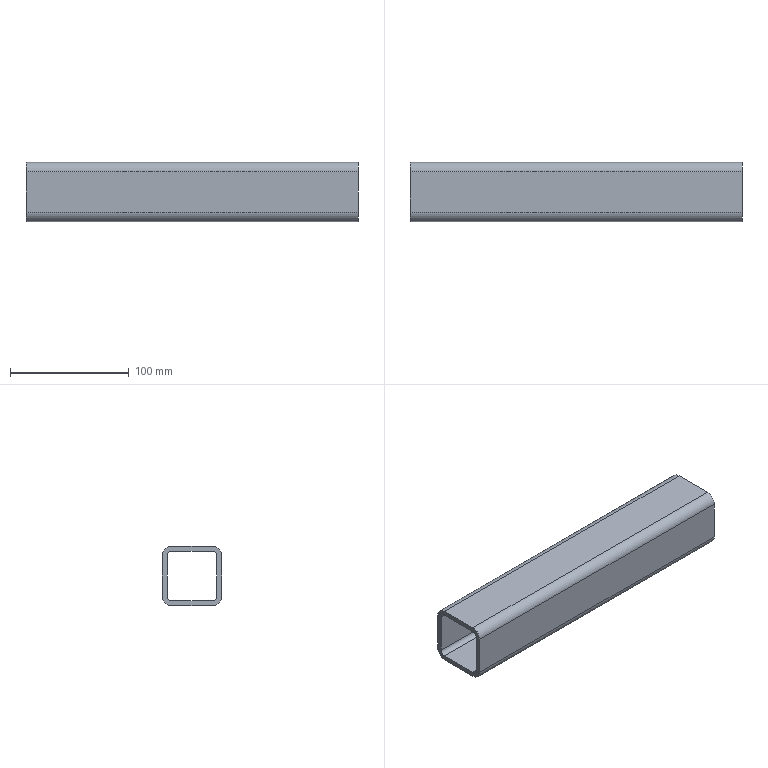Part | STEP file | 50X50X280 square tube_default<machined> | 1 solid | 18 faces | box 280 x 50 x 50 mm | volume 194543 mm3 | plane 10 | cylinder 8 | commonest cylinder face diameters 8 x4 16 x4
STEP:
#1=CARTESIAN_POINT('',(0.,0.,0.));
#2=DIRECTION('',(0.,0.,1.));
#3=DIRECTION('',(1.,0.,0.));
#4=AXIS2_PLACEMENT_3D('',#1,#2,#3);
#5=CARTESIAN_POINT('',(-140.,25.,17.));
#6=VERTEX_POINT('',#5);
#7=CARTESIAN_POINT('',(-140.,17.,25.));
#8=VERTEX_POINT('',#7);
#9=CARTESIAN_POINT('',(-140.,17.,17.));
#10=DIRECTION('',(1.,0.,0.));
#11=DIRECTION('',(0.,1.,0.));
#12=AXIS2_PLACEMENT_3D('',#9,#10,#11);
#13=CIRCLE('',#12,8.);
#14=CARTESIAN_POINT('',(140.,17.,17.));
#15=DIRECTION('',(-1.,0.,0.));
#16=DIRECTION('',(0.,-1.,0.));
#17=AXIS2_PLACEMENT_3D('',#14,#15,#16);
#18=CYLINDRICAL_SURFACE('',#17,8.);
#19=CARTESIAN_POINT('',(3.142,280.));
#20=DIRECTION('',(-1.,0.));
#21=VECTOR('',#20,1.);
#22=LINE('',#19,#21);
#23=(GEOMETRIC_REPRESENTATION_CONTEXT(2)PARAMETRIC_REPRESENTATION_CONTEXT()REPRESENTATION_CONTEXT('',''));
#24=DEFINITIONAL_REPRESENTATION('',(#22),#23);
#25=PCURVE('',#18,#24);
#26=CARTESIAN_POINT('',(-140.,17.,17.));
#27=DIRECTION('',(1.,0.,0.));
#28=DIRECTION('',(0.,1.,0.));
#29=AXIS2_PLACEMENT_3D('',#26,#27,#28);
#30=PLANE('',#29);
#31=CARTESIAN_POINT('',(0.,0.));
#32=DIRECTION('',(1.,0.));
#33=AXIS2_PLACEMENT_2D('',#31,#32);
#34=CIRCLE('',#33,8.);
#35=(GEOMETRIC_REPRESENTATION_CONTEXT(2)PARAMETRIC_REPRESENTATION_CONTEXT()REPRESENTATION_CONTEXT('',''));
#36=DEFINITIONAL_REPRESENTATION('',(#34),#35);
#37=PCURVE('',#30,#36);
#38=SURFACE_CURVE('',#13,(#25,#37),.PCURVE_S1.);
#39=EDGE_CURVE('',#6,#8,#38,.T.);
#40=ORIENTED_EDGE('',*,*,#39,.T.);
#41=CARTESIAN_POINT('',(140.,17.,25.));
#42=VERTEX_POINT('',#41);
#43=CARTESIAN_POINT('',(140.,17.,25.));
#44=DIRECTION('',(-1.,0.,0.));
#45=VECTOR('',#44,1.);
#46=LINE('',#43,#45);
#47=CARTESIAN_POINT('',(1.571,0.));
#48=DIRECTION('',(0.,1.));
#49=VECTOR('',#48,1.);
#50=LINE('',#47,#49);
#51=(GEOMETRIC_REPRESENTATION_CONTEXT(2)PARAMETRIC_REPRESENTATION_CONTEXT()REPRESENTATION_CONTEXT('',''));
#52=DEFINITIONAL_REPRESENTATION('',(#50),#51);
#53=PCURVE('',#18,#52);
#54=CARTESIAN_POINT('',(140.,17.,25.));
#55=DIRECTION('',(0.,0.,-1.));
#56=DIRECTION('',(-1.,0.,0.));
#57=AXIS2_PLACEMENT_3D('',#54,#55,#56);
#58=PLANE('',#57);
#59=CARTESIAN_POINT('',(0.,0.));
#60=DIRECTION('',(1.,0.));
#61=VECTOR('',#60,1.);
#62=LINE('',#59,#61);
#63=(GEOMETRIC_REPRESENTATION_CONTEXT(2)PARAMETRIC_REPRESENTATION_CONTEXT()REPRESENTATION_CONTEXT('',''));
#64=DEFINITIONAL_REPRESENTATION('',(#62),#63);
#65=PCURVE('',#58,#64);
#66=SURFACE_CURVE('',#46,(#53,#65),.PCURVE_S1.);
#67=EDGE_CURVE('',#42,#8,#66,.T.);
#68=ORIENTED_EDGE('',*,*,#67,.F.);
#69=CARTESIAN_POINT('',(140.,25.,17.));
#70=VERTEX_POINT('',#69);
#71=CARTESIAN_POINT('',(140.,17.,17.));
#72=DIRECTION('',(1.,0.,0.));
#73=DIRECTION('',(0.,1.,0.));
#74=AXIS2_PLACEMENT_3D('',#71,#72,#73);
#75=CIRCLE('',#74,8.);
#76=CARTESIAN_POINT('',(3.142,0.));
#77=DIRECTION('',(-1.,0.));
#78=VECTOR('',#77,1.);
#79=LINE('',#76,#78);
#80=(GEOMETRIC_REPRESENTATION_CONTEXT(2)PARAMETRIC_REPRESENTATION_CONTEXT()REPRESENTATION_CONTEXT('',''));
#81=DEFINITIONAL_REPRESENTATION('',(#79),#80);
#82=PCURVE('',#18,#81);
#83=CARTESIAN_POINT('',(140.,17.,17.));
#84=DIRECTION('',(1.,0.,0.));
#85=DIRECTION('',(0.,1.,0.));
#86=AXIS2_PLACEMENT_3D('',#83,#84,#85);
#87=PLANE('',#86);
#88=CARTESIAN_POINT('',(0.,0.));
#89=DIRECTION('',(1.,0.));
#90=AXIS2_PLACEMENT_2D('',#88,#89);
#91=CIRCLE('',#90,8.);
#92=(GEOMETRIC_REPRESENTATION_CONTEXT(2)PARAMETRIC_REPRESENTATION_CONTEXT()REPRESENTATION_CONTEXT('',''));
#93=DEFINITIONAL_REPRESENTATION('',(#91),#92);
#94=PCURVE('',#87,#93);
#95=SURFACE_CURVE('',#75,(#82,#94),.PCURVE_S1.);
#96=EDGE_CURVE('',#70,#42,#95,.T.);
#97=ORIENTED_EDGE('',*,*,#96,.F.);
#98=CARTESIAN_POINT('',(140.,25.,17.));
#99=DIRECTION('',(-1.,0.,0.));
#100=VECTOR('',#99,1.);
#101=LINE('',#98,#100);
#102=CARTESIAN_POINT('',(3.142,0.));
#103=DIRECTION('',(0.,1.));
#104=VECTOR('',#103,1.);
#105=LINE('',#102,#104);
#106=(GEOMETRIC_REPRESENTATION_CONTEXT(2)PARAMETRIC_REPRESENTATION_CONTEXT()REPRESENTATION_CONTEXT('',''));
#107=DEFINITIONAL_REPRESENTATION('',(#105),#106);
#108=PCURVE('',#18,#107);
#109=CARTESIAN_POINT('',(140.,25.,17.));
#110=DIRECTION('',(0.,-1.,0.));
#111=DIRECTION('',(1.,0.,0.));
#112=AXIS2_PLACEMENT_3D('',#109,#110,#111);
#113=PLANE('',#112);
#114=CARTESIAN_POINT('',(0.,0.));
#115=DIRECTION('',(-1.,0.));
#116=VECTOR('',#115,1.);
#117=LINE('',#114,#116);
#118=(GEOMETRIC_REPRESENTATION_CONTEXT(2)PARAMETRIC_REPRESENTATION_CONTEXT()REPRESENTATION_CONTEXT('',''));
#119=DEFINITIONAL_REPRESENTATION('',(#117),#118);
#120=PCURVE('',#113,#119);
#121=SURFACE_CURVE('',#101,(#108,#120),.PCURVE_S1.);
#122=EDGE_CURVE('',#70,#6,#121,.T.);
#123=ORIENTED_EDGE('',*,*,#122,.T.);
#124=EDGE_LOOP('',(#40,#68,#97,#123));
#125=FACE_BOUND('',#124,.T.);
#126=ADVANCED_FACE('',(#125),#18,.T.);
#127=CARTESIAN_POINT('',(-140.,-17.,25.));
#128=VERTEX_POINT('',#127);
#129=CARTESIAN_POINT('',(-140.,17.,25.));
#130=DIRECTION('',(0.,-1.,0.));
#131=VECTOR('',#130,1.);
#132=LINE('',#129,#131);
#133=CARTESIAN_POINT('',(280.,0.));
#134=DIRECTION('',(0.,-1.));
#135=VECTOR('',#134,1.);
#136=LINE('',#133,#135);
#137=(GEOMETRIC_REPRESENTATION_CONTEXT(2)PARAMETRIC_REPRESENTATION_CONTEXT()REPRESENTATION_CONTEXT('',''));
#138=DEFINITIONAL_REPRESENTATION('',(#136),#137);
#139=PCURVE('',#58,#138);
#140=CARTESIAN_POINT('',(0.,8.));
#141=DIRECTION('',(-1.,0.));
#142=VECTOR('',#141,1.);
#143=LINE('',#140,#142);
#144=(GEOMETRIC_REPRESENTATION_CONTEXT(2)PARAMETRIC_REPRESENTATION_CONTEXT()REPRESENTATION_CONTEXT('',''));
#145=DEFINITIONAL_REPRESENTATION('',(#143),#144);
#146=PCURVE('',#30,#145);
#147=SURFACE_CURVE('',#132,(#139,#146),.PCURVE_S1.);
#148=EDGE_CURVE('',#8,#128,#147,.T.);
#149=ORIENTED_EDGE('',*,*,#148,.T.);
#150=CARTESIAN_POINT('',(140.,-17.,25.));
#151=VERTEX_POINT('',#150);
#152=CARTESIAN_POINT('',(140.,-17.,25.));
#153=DIRECTION('',(-1.,0.,0.));
#154=VECTOR('',#153,1.);
#155=LINE('',#152,#154);
#156=CARTESIAN_POINT('',(0.,-34.));
#157=DIRECTION('',(1.,0.));
#158=VECTOR('',#157,1.);
#159=LINE('',#156,#158);
#160=(GEOMETRIC_REPRESENTATION_CONTEXT(2)PARAMETRIC_REPRESENTATION_CONTEXT()REPRESENTATION_CONTEXT('',''));
#161=DEFINITIONAL_REPRESENTATION('',(#159),#160);
#162=PCURVE('',#58,#161);
#163=CARTESIAN_POINT('',(140.,-17.,17.));
#164=DIRECTION('',(-1.,0.,0.));
#165=DIRECTION('',(0.,-1.,0.));
#166=AXIS2_PLACEMENT_3D('',#163,#164,#165);
#167=CYLINDRICAL_SURFACE('',#166,8.);
#168=CARTESIAN_POINT('',(1.571,0.));
#169=DIRECTION('',(0.,1.));
#170=VECTOR('',#169,1.);
#171=LINE('',#168,#170);
#172=(GEOMETRIC_REPRESENTATION_CONTEXT(2)PARAMETRIC_REPRESENTATION_CONTEXT()REPRESENTATION_CONTEXT('',''));
#173=DEFINITIONAL_REPRESENTATION('',(#171),#172);
#174=PCURVE('',#167,#173);
#175=SURFACE_CURVE('',#155,(#162,#174),.PCURVE_S1.);
#176=EDGE_CURVE('',#151,#128,#175,.T.);
#177=ORIENTED_EDGE('',*,*,#176,.F.);
#178=CARTESIAN_POINT('',(140.,17.,25.));
#179=DIRECTION('',(0.,-1.,0.));
#180=VECTOR('',#179,1.);
#181=LINE('',#178,#180);
#182=CARTESIAN_POINT('',(0.,0.));
#183=DIRECTION('',(0.,-1.));
#184=VECTOR('',#183,1.);
#185=LINE('',#182,#184);
#186=(GEOMETRIC_REPRESENTATION_CONTEXT(2)PARAMETRIC_REPRESENTATION_CONTEXT()REPRESENTATION_CONTEXT('',''));
#187=DEFINITIONAL_REPRESENTATION('',(#185),#186);
#188=PCURVE('',#58,#187);
#189=CARTESIAN_POINT('',(0.,8.));
#190=DIRECTION('',(-1.,0.));
#191=VECTOR('',#190,1.);
#192=LINE('',#189,#191);
#193=(GEOMETRIC_REPRESENTATION_CONTEXT(2)PARAMETRIC_REPRESENTATION_CONTEXT()REPRESENTATION_CONTEXT('',''));
#194=DEFINITIONAL_REPRESENTATION('',(#192),#193);
#195=PCURVE('',#87,#194);
#196=SURFACE_CURVE('',#181,(#188,#195),.PCURVE_S1.);
#197=EDGE_CURVE('',#42,#151,#196,.T.);
#198=ORIENTED_EDGE('',*,*,#197,.F.);
#199=ORIENTED_EDGE('',*,*,#67,.T.);
#200=EDGE_LOOP('',(#149,#177,#198,#199));
#201=FACE_BOUND('',#200,.T.);
#202=ADVANCED_FACE('',(#201),#58,.F.);
#203=CARTESIAN_POINT('',(-140.,-25.,17.));
#204=VERTEX_POINT('',#203);
#205=CARTESIAN_POINT('',(-140.,-17.,17.));
#206=DIRECTION('',(1.,0.,0.));
#207=DIRECTION('',(0.,1.,0.));
#208=AXIS2_PLACEMENT_3D('',#205,#206,#207);
#209=CIRCLE('',#208,8.);
#210=CARTESIAN_POINT('',(3.142,280.));
#211=DIRECTION('',(-1.,0.));
#212=VECTOR('',#211,1.);
#213=LINE('',#210,#212);
#214=(GEOMETRIC_REPRESENTATION_CONTEXT(2)PARAMETRIC_REPRESENTATION_CONTEXT()REPRESENTATION_CONTEXT('',''));
#215=DEFINITIONAL_REPRESENTATION('',(#213),#214);
#216=PCURVE('',#167,#215);
#217=CARTESIAN_POINT('',(-34.,0.));
#218=DIRECTION('',(1.,0.));
#219=AXIS2_PLACEMENT_2D('',#217,#218);
#220=CIRCLE('',#219,8.);
#221=(GEOMETRIC_REPRESENTATION_CONTEXT(2)PARAMETRIC_REPRESENTATION_CONTEXT()REPRESENTATION_CONTEXT('',''));
#222=DEFINITIONAL_REPRESENTATION('',(#220),#221);
#223=PCURVE('',#30,#222);
#224=SURFACE_CURVE('',#209,(#216,#223),.PCURVE_S1.);
#225=EDGE_CURVE('',#128,#204,#224,.T.);
#226=ORIENTED_EDGE('',*,*,#225,.T.);
#227=CARTESIAN_POINT('',(140.,-25.,17.));
#228=VERTEX_POINT('',#227);
#229=CARTESIAN_POINT('',(140.,-25.,17.));
#230=DIRECTION('',(-1.,0.,0.));
#231=VECTOR('',#230,1.);
#232=LINE('',#229,#231);
#233=CARTESIAN_POINT('',(0.,0.));
#234=DIRECTION('',(0.,1.));
#235=VECTOR('',#234,1.);
#236=LINE('',#233,#235);
#237=(GEOMETRIC_REPRESENTATION_CONTEXT(2)PARAMETRIC_REPRESENTATION_CONTEXT()REPRESENTATION_CONTEXT('',''));
#238=DEFINITIONAL_REPRESENTATION('',(#236),#237);
#239=PCURVE('',#167,#238);
#240=CARTESIAN_POINT('',(140.,-25.,-17.));
#241=DIRECTION('',(0.,1.,0.));
#242=DIRECTION('',(-1.,0.,0.));
#243=AXIS2_PLACEMENT_3D('',#240,#241,#242);
#244=PLANE('',#243);
#245=CARTESIAN_POINT('',(0.,34.));
#246=DIRECTION('',(1.,0.));
#247=VECTOR('',#246,1.);
#248=LINE('',#245,#247);
#249=(GEOMETRIC_REPRESENTATION_CONTEXT(2)PARAMETRIC_REPRESENTATION_CONTEXT()REPRESENTATION_CONTEXT('',''));
#250=DEFINITIONAL_REPRESENTATION('',(#248),#249);
#251=PCURVE('',#244,#250);
#252=SURFACE_CURVE('',#232,(#239,#251),.PCURVE_S1.);
#253=EDGE_CURVE('',#228,#204,#252,.T.);
#254=ORIENTED_EDGE('',*,*,#253,.F.);
#255=CARTESIAN_POINT('',(140.,-17.,17.));
#256=DIRECTION('',(1.,0.,0.));
#257=DIRECTION('',(0.,1.,0.));
#258=AXIS2_PLACEMENT_3D('',#255,#256,#257);
#259=CIRCLE('',#258,8.);
#260=CARTESIAN_POINT('',(3.142,0.));
#261=DIRECTION('',(-1.,0.));
#262=VECTOR('',#261,1.);
#263=LINE('',#260,#262);
#264=(GEOMETRIC_REPRESENTATION_CONTEXT(2)PARAMETRIC_REPRESENTATION_CONTEXT()REPRESENTATION_CONTEXT('',''));
#265=DEFINITIONAL_REPRESENTATION('',(#263),#264);
#266=PCURVE('',#167,#265);
#267=CARTESIAN_POINT('',(-34.,0.));
#268=DIRECTION('',(1.,0.));
#269=AXIS2_PLACEMENT_2D('',#267,#268);
#270=CIRCLE('',#269,8.);
#271=(GEOMETRIC_REPRESENTATION_CONTEXT(2)PARAMETRIC_REPRESENTATION_CONTEXT()REPRESENTATION_CONTEXT('',''));
#272=DEFINITIONAL_REPRESENTATION('',(#270),#271);
#273=PCURVE('',#87,#272);
#274=SURFACE_CURVE('',#259,(#266,#273),.PCURVE_S1.);
#275=EDGE_CURVE('',#151,#228,#274,.T.);
#276=ORIENTED_EDGE('',*,*,#275,.F.);
#277=ORIENTED_EDGE('',*,*,#176,.T.);
#278=EDGE_LOOP('',(#226,#254,#276,#277));
#279=FACE_BOUND('',#278,.T.);
#280=ADVANCED_FACE('',(#279),#167,.T.);
#281=CARTESIAN_POINT('',(-140.,-25.,-17.));
#282=VERTEX_POINT('',#281);
#283=CARTESIAN_POINT('',(-140.,-25.,-17.));
#284=DIRECTION('',(0.,0.,-1.));
#285=VECTOR('',#284,1.);
#286=LINE('',#283,#285);
#287=CARTESIAN_POINT('',(280.,0.));
#288=DIRECTION('',(0.,-1.));
#289=VECTOR('',#288,1.);
#290=LINE('',#287,#289);
#291=(GEOMETRIC_REPRESENTATION_CONTEXT(2)PARAMETRIC_REPRESENTATION_CONTEXT()REPRESENTATION_CONTEXT('',''));
#292=DEFINITIONAL_REPRESENTATION('',(#290),#291);
#293=PCURVE('',#244,#292);
#294=CARTESIAN_POINT('',(-42.,-34.));
#295=DIRECTION('',(0.,-1.));
#296=VECTOR('',#295,1.);
#297=LINE('',#294,#296);
#298=(GEOMETRIC_REPRESENTATION_CONTEXT(2)PARAMETRIC_REPRESENTATION_CONTEXT()REPRESENTATION_CONTEXT('',''));
#299=DEFINITIONAL_REPRESENTATION('',(#297),#298);
#300=PCURVE('',#30,#299);
#301=SURFACE_CURVE('',#286,(#293,#300),.PCURVE_S1.);
#302=EDGE_CURVE('',#204,#282,#301,.T.);
#303=ORIENTED_EDGE('',*,*,#302,.T.);
#304=CARTESIAN_POINT('',(140.,-25.,-17.));
#305=VERTEX_POINT('',#304);
#306=CARTESIAN_POINT('',(140.,-25.,-17.));
#307=DIRECTION('',(-1.,0.,0.));
#308=VECTOR('',#307,1.);
#309=LINE('',#306,#308);
#310=CARTESIAN_POINT('',(0.,0.));
#311=DIRECTION('',(1.,0.));
#312=VECTOR('',#311,1.);
#313=LINE('',#310,#312);
#314=(GEOMETRIC_REPRESENTATION_CONTEXT(2)PARAMETRIC_REPRESENTATION_CONTEXT()REPRESENTATION_CONTEXT('',''));
#315=DEFINITIONAL_REPRESENTATION('',(#313),#314);
#316=PCURVE('',#244,#315);
#317=CARTESIAN_POINT('',(140.,-17.,-17.));
#318=DIRECTION('',(-1.,0.,0.));
#319=DIRECTION('',(0.,-1.,0.));
#320=AXIS2_PLACEMENT_3D('',#317,#318,#319);
#321=CYLINDRICAL_SURFACE('',#320,8.);
#322=CARTESIAN_POINT('',(6.283,0.));
#323=DIRECTION('',(0.,1.));
#324=VECTOR('',#323,1.);
#325=LINE('',#322,#324);
#326=(GEOMETRIC_REPRESENTATION_CONTEXT(2)PARAMETRIC_REPRESENTATION_CONTEXT()REPRESENTATION_CONTEXT('',''));
#327=DEFINITIONAL_REPRESENTATION('',(#325),#326);
#328=PCURVE('',#321,#327);
#329=SURFACE_CURVE('',#309,(#316,#328),.PCURVE_S1.);
#330=EDGE_CURVE('',#305,#282,#329,.T.);
#331=ORIENTED_EDGE('',*,*,#330,.F.);
#332=CARTESIAN_POINT('',(140.,-25.,-17.));
#333=DIRECTION('',(0.,0.,-1.));
#334=VECTOR('',#333,1.);
#335=LINE('',#332,#334);
#336=CARTESIAN_POINT('',(0.,0.));
#337=DIRECTION('',(0.,-1.));
#338=VECTOR('',#337,1.);
#339=LINE('',#336,#338);
#340=(GEOMETRIC_REPRESENTATION_CONTEXT(2)PARAMETRIC_REPRESENTATION_CONTEXT()REPRESENTATION_CONTEXT('',''));
#341=DEFINITIONAL_REPRESENTATION('',(#339),#340);
#342=PCURVE('',#244,#341);
#343=CARTESIAN_POINT('',(-42.,-34.));
#344=DIRECTION('',(0.,-1.));
#345=VECTOR('',#344,1.);
#346=LINE('',#343,#345);
#347=(GEOMETRIC_REPRESENTATION_CONTEXT(2)PARAMETRIC_REPRESENTATION_CONTEXT()REPRESENTATION_CONTEXT('',''));
#348=DEFINITIONAL_REPRESENTATION('',(#346),#347);
#349=PCURVE('',#87,#348);
#350=SURFACE_CURVE('',#335,(#342,#349),.PCURVE_S1.);
#351=EDGE_CURVE('',#228,#305,#350,.T.);
#352=ORIENTED_EDGE('',*,*,#351,.F.);
#353=ORIENTED_EDGE('',*,*,#253,.T.);
#354=EDGE_LOOP('',(#303,#331,#352,#353));
#355=FACE_BOUND('',#354,.T.);
#356=ADVANCED_FACE('',(#355),#244,.F.);
#357=CARTESIAN_POINT('',(-140.,-17.,-25.));
#358=VERTEX_POINT('',#357);
#359=CARTESIAN_POINT('',(-140.,-17.,-17.));
#360=DIRECTION('',(1.,0.,0.));
#361=DIRECTION('',(0.,1.,0.));
#362=AXIS2_PLACEMENT_3D('',#359,#360,#361);
#363=CIRCLE('',#362,8.);
#364=CARTESIAN_POINT('',(9.425,280.));
#365=DIRECTION('',(-1.,0.));
#366=VECTOR('',#365,1.);
#367=LINE('',#364,#366);
#368=(GEOMETRIC_REPRESENTATION_CONTEXT(2)PARAMETRIC_REPRESENTATION_CONTEXT()REPRESENTATION_CONTEXT('',''));
#369=DEFINITIONAL_REPRESENTATION('',(#367),#368);
#370=PCURVE('',#321,#369);
#371=CARTESIAN_POINT('',(-34.,-34.));
#372=DIRECTION('',(1.,0.));
#373=AXIS2_PLACEMENT_2D('',#371,#372);
#374=CIRCLE('',#373,8.);
#375=(GEOMETRIC_REPRESENTATION_CONTEXT(2)PARAMETRIC_REPRESENTATION_CONTEXT()REPRESENTATION_CONTEXT('',''));
#376=DEFINITIONAL_REPRESENTATION('',(#374),#375);
#377=PCURVE('',#30,#376);
#378=SURFACE_CURVE('',#363,(#370,#377),.PCURVE_S1.);
#379=EDGE_CURVE('',#282,#358,#378,.T.);
#380=ORIENTED_EDGE('',*,*,#379,.T.);
#381=CARTESIAN_POINT('',(140.,-17.,-25.));
#382=VERTEX_POINT('',#381);
#383=CARTESIAN_POINT('',(140.,-17.,-25.));
#384=DIRECTION('',(-1.,0.,0.));
#385=VECTOR('',#384,1.);
#386=LINE('',#383,#385);
#387=CARTESIAN_POINT('',(4.712,0.));
#388=DIRECTION('',(0.,1.));
#389=VECTOR('',#388,1.);
#390=LINE('',#387,#389);
#391=(GEOMETRIC_REPRESENTATION_CONTEXT(2)PARAMETRIC_REPRESENTATION_CONTEXT()REPRESENTATION_CONTEXT('',''));
#392=DEFINITIONAL_REPRESENTATION('',(#390),#391);
#393=PCURVE('',#321,#392);
#394=CARTESIAN_POINT('',(140.,-17.,-25.));
#395=DIRECTION('',(0.,0.,1.));
#396=DIRECTION('',(1.,0.,0.));
#397=AXIS2_PLACEMENT_3D('',#394,#395,#396);
#398=PLANE('',#397);
#399=CARTESIAN_POINT('',(0.,0.));
#400=DIRECTION('',(-1.,0.));
#401=VECTOR('',#400,1.);
#402=LINE('',#399,#401);
#403=(GEOMETRIC_REPRESENTATION_CONTEXT(2)PARAMETRIC_REPRESENTATION_CONTEXT()REPRESENTATION_CONTEXT('',''));
#404=DEFINITIONAL_REPRESENTATION('',(#402),#403);
#405=PCURVE('',#398,#404);
#406=SURFACE_CURVE('',#386,(#393,#405),.PCURVE_S1.);
#407=EDGE_CURVE('',#382,#358,#406,.T.);
#408=ORIENTED_EDGE('',*,*,#407,.F.);
#409=CARTESIAN_POINT('',(140.,-17.,-17.));
#410=DIRECTION('',(1.,0.,0.));
#411=DIRECTION('',(0.,1.,0.));
#412=AXIS2_PLACEMENT_3D('',#409,#410,#411);
#413=CIRCLE('',#412,8.);
#414=CARTESIAN_POINT('',(9.425,0.));
#415=DIRECTION('',(-1.,0.));
#416=VECTOR('',#415,1.);
#417=LINE('',#414,#416);
#418=(GEOMETRIC_REPRESENTATION_CONTEXT(2)PARAMETRIC_REPRESENTATION_CONTEXT()REPRESENTATION_CONTEXT('',''));
#419=DEFINITIONAL_REPRESENTATION('',(#417),#418);
#420=PCURVE('',#321,#419);
#421=CARTESIAN_POINT('',(-34.,-34.));
#422=DIRECTION('',(1.,0.));
#423=AXIS2_PLACEMENT_2D('',#421,#422);
#424=CIRCLE('',#423,8.);
#425=(GEOMETRIC_REPRESENTATION_CONTEXT(2)PARAMETRIC_REPRESENTATION_CONTEXT()REPRESENTATION_CONTEXT('',''));
#426=DEFINITIONAL_REPRESENTATION('',(#424),#425);
#427=PCURVE('',#87,#426);
#428=SURFACE_CURVE('',#413,(#420,#427),.PCURVE_S1.);
#429=EDGE_CURVE('',#305,#382,#428,.T.);
#430=ORIENTED_EDGE('',*,*,#429,.F.);
#431=ORIENTED_EDGE('',*,*,#330,.T.);
#432=EDGE_LOOP('',(#380,#408,#430,#431));
#433=FACE_BOUND('',#432,.T.);
#434=ADVANCED_FACE('',(#433),#321,.T.);
#435=CARTESIAN_POINT('',(-140.,17.,-25.));
#436=VERTEX_POINT('',#435);
#437=CARTESIAN_POINT('',(-140.,-17.,-25.));
#438=DIRECTION('',(0.,1.,0.));
#439=VECTOR('',#438,1.);
#440=LINE('',#437,#439);
#441=CARTESIAN_POINT('',(-280.,0.));
#442=DIRECTION('',(0.,1.));
#443=VECTOR('',#442,1.);
#444=LINE('',#441,#443);
#445=(GEOMETRIC_REPRESENTATION_CONTEXT(2)PARAMETRIC_REPRESENTATION_CONTEXT()REPRESENTATION_CONTEXT('',''));
#446=DEFINITIONAL_REPRESENTATION('',(#444),#445);
#447=PCURVE('',#398,#446);
#448=CARTESIAN_POINT('',(-34.,-42.));
#449=DIRECTION('',(1.,0.));
#450=VECTOR('',#449,1.);
#451=LINE('',#448,#450);
#452=(GEOMETRIC_REPRESENTATION_CONTEXT(2)PARAMETRIC_REPRESENTATION_CONTEXT()REPRESENTATION_CONTEXT('',''));
#453=DEFINITIONAL_REPRESENTATION('',(#451),#452);
#454=PCURVE('',#30,#453);
#455=SURFACE_CURVE('',#440,(#447,#454),.PCURVE_S1.);
#456=EDGE_CURVE('',#358,#436,#455,.T.);
#457=ORIENTED_EDGE('',*,*,#456,.T.);
#458=CARTESIAN_POINT('',(140.,17.,-25.));
#459=VERTEX_POINT('',#458);
#460=CARTESIAN_POINT('',(140.,17.,-25.));
#461=DIRECTION('',(-1.,0.,0.));
#462=VECTOR('',#461,1.);
#463=LINE('',#460,#462);
#464=CARTESIAN_POINT('',(0.,34.));
#465=DIRECTION('',(-1.,0.));
#466=VECTOR('',#465,1.);
#467=LINE('',#464,#466);
#468=(GEOMETRIC_REPRESENTATION_CONTEXT(2)PARAMETRIC_REPRESENTATION_CONTEXT()REPRESENTATION_CONTEXT('',''));
#469=DEFINITIONAL_REPRESENTATION('',(#467),#468);
#470=PCURVE('',#398,#469);
#471=CARTESIAN_POINT('',(140.,17.,-17.));
#472=DIRECTION('',(-1.,0.,0.));
#473=DIRECTION('',(0.,-1.,0.));
#474=AXIS2_PLACEMENT_3D('',#471,#472,#473);
#475=CYLINDRICAL_SURFACE('',#474,8.);
#476=CARTESIAN_POINT('',(4.712,0.));
#477=DIRECTION('',(0.,1.));
#478=VECTOR('',#477,1.);
#479=LINE('',#476,#478);
#480=(GEOMETRIC_REPRESENTATION_CONTEXT(2)PARAMETRIC_REPRESENTATION_CONTEXT()REPRESENTATION_CONTEXT('',''));
#481=DEFINITIONAL_REPRESENTATION('',(#479),#480);
#482=PCURVE('',#475,#481);
#483=SURFACE_CURVE('',#463,(#470,#482),.PCURVE_S1.);
#484=EDGE_CURVE('',#459,#436,#483,.T.);
#485=ORIENTED_EDGE('',*,*,#484,.F.);
#486=CARTESIAN_POINT('',(140.,-17.,-25.));
#487=DIRECTION('',(0.,1.,0.));
#488=VECTOR('',#487,1.);
#489=LINE('',#486,#488);
#490=CARTESIAN_POINT('',(0.,0.));
#491=DIRECTION('',(0.,1.));
#492=VECTOR('',#491,1.);
#493=LINE('',#490,#492);
#494=(GEOMETRIC_REPRESENTATION_CONTEXT(2)PARAMETRIC_REPRESENTATION_CONTEXT()REPRESENTATION_CONTEXT('',''));
#495=DEFINITIONAL_REPRESENTATION('',(#493),#494);
#496=PCURVE('',#398,#495);
#497=CARTESIAN_POINT('',(-34.,-42.));
#498=DIRECTION('',(1.,0.));
#499=VECTOR('',#498,1.);
#500=LINE('',#497,#499);
#501=(GEOMETRIC_REPRESENTATION_CONTEXT(2)PARAMETRIC_REPRESENTATION_CONTEXT()REPRESENTATION_CONTEXT('',''));
#502=DEFINITIONAL_REPRESENTATION('',(#500),#501);
#503=PCURVE('',#87,#502);
#504=SURFACE_CURVE('',#489,(#496,#503),.PCURVE_S1.);
#505=EDGE_CURVE('',#382,#459,#504,.T.);
#506=ORIENTED_EDGE('',*,*,#505,.F.);
#507=ORIENTED_EDGE('',*,*,#407,.T.);
#508=EDGE_LOOP('',(#457,#485,#506,#507));
#509=FACE_BOUND('',#508,.T.);
#510=ADVANCED_FACE('',(#509),#398,.F.);
#511=CARTESIAN_POINT('',(-140.,25.,-17.));
#512=VERTEX_POINT('',#511);
#513=CARTESIAN_POINT('',(-140.,17.,-17.));
#514=DIRECTION('',(1.,0.,0.));
#515=DIRECTION('',(0.,1.,0.));
#516=AXIS2_PLACEMENT_3D('',#513,#514,#515);
#517=CIRCLE('',#516,8.);
#518=CARTESIAN_POINT('',(9.425,280.));
#519=DIRECTION('',(-1.,0.));
#520=VECTOR('',#519,1.);
#521=LINE('',#518,#520);
#522=(GEOMETRIC_REPRESENTATION_CONTEXT(2)PARAMETRIC_REPRESENTATION_CONTEXT()REPRESENTATION_CONTEXT('',''));
#523=DEFINITIONAL_REPRESENTATION('',(#521),#522);
#524=PCURVE('',#475,#523);
#525=CARTESIAN_POINT('',(0.,-34.));
#526=DIRECTION('',(1.,0.));
#527=AXIS2_PLACEMENT_2D('',#525,#526);
#528=CIRCLE('',#527,8.);
#529=(GEOMETRIC_REPRESENTATION_CONTEXT(2)PARAMETRIC_REPRESENTATION_CONTEXT()REPRESENTATION_CONTEXT('',''));
#530=DEFINITIONAL_REPRESENTATION('',(#528),#529);
#531=PCURVE('',#30,#530);
#532=SURFACE_CURVE('',#517,(#524,#531),.PCURVE_S1.);
#533=EDGE_CURVE('',#436,#512,#532,.T.);
#534=ORIENTED_EDGE('',*,*,#533,.T.);
#535=CARTESIAN_POINT('',(140.,25.,-17.));
#536=VERTEX_POINT('',#535);
#537=CARTESIAN_POINT('',(140.,25.,-17.));
#538=DIRECTION('',(-1.,0.,0.));
#539=VECTOR('',#538,1.);
#540=LINE('',#537,#539);
#541=CARTESIAN_POINT('',(3.142,0.));
#542=DIRECTION('',(0.,1.));
#543=VECTOR('',#542,1.);
#544=LINE('',#541,#543);
#545=(GEOMETRIC_REPRESENTATION_CONTEXT(2)PARAMETRIC_REPRESENTATION_CONTEXT()REPRESENTATION_CONTEXT('',''));
#546=DEFINITIONAL_REPRESENTATION('',(#544),#545);
#547=PCURVE('',#475,#546);
#548=CARTESIAN_POINT('',(0.,-34.));
#549=DIRECTION('',(-1.,0.));
#550=VECTOR('',#549,1.);
#551=LINE('',#548,#550);
#552=(GEOMETRIC_REPRESENTATION_CONTEXT(2)PARAMETRIC_REPRESENTATION_CONTEXT()REPRESENTATION_CONTEXT('',''));
#553=DEFINITIONAL_REPRESENTATION('',(#551),#552);
#554=PCURVE('',#113,#553);
#555=SURFACE_CURVE('',#540,(#547,#554),.PCURVE_S1.);
#556=EDGE_CURVE('',#536,#512,#555,.T.);
#557=ORIENTED_EDGE('',*,*,#556,.F.);
#558=CARTESIAN_POINT('',(140.,17.,-17.));
#559=DIRECTION('',(1.,0.,0.));
#560=DIRECTION('',(0.,1.,0.));
#561=AXIS2_PLACEMENT_3D('',#558,#559,#560);
#562=CIRCLE('',#561,8.);
#563=CARTESIAN_POINT('',(9.425,0.));
#564=DIRECTION('',(-1.,0.));
#565=VECTOR('',#564,1.);
#566=LINE('',#563,#565);
#567=(GEOMETRIC_REPRESENTATION_CONTEXT(2)PARAMETRIC_REPRESENTATION_CONTEXT()REPRESENTATION_CONTEXT('',''));
#568=DEFINITIONAL_REPRESENTATION('',(#566),#567);
#569=PCURVE('',#475,#568);
#570=CARTESIAN_POINT('',(0.,-34.));
#571=DIRECTION('',(1.,0.));
#572=AXIS2_PLACEMENT_2D('',#570,#571);
#573=CIRCLE('',#572,8.);
#574=(GEOMETRIC_REPRESENTATION_CONTEXT(2)PARAMETRIC_REPRESENTATION_CONTEXT()REPRESENTATION_CONTEXT('',''));
#575=DEFINITIONAL_REPRESENTATION('',(#573),#574);
#576=PCURVE('',#87,#575);
#577=SURFACE_CURVE('',#562,(#569,#576),.PCURVE_S1.);
#578=EDGE_CURVE('',#459,#536,#577,.T.);
#579=ORIENTED_EDGE('',*,*,#578,.F.);
#580=ORIENTED_EDGE('',*,*,#484,.T.);
#581=EDGE_LOOP('',(#534,#557,#579,#580));
#582=FACE_BOUND('',#581,.T.);
#583=ADVANCED_FACE('',(#582),#475,.T.);
#584=CARTESIAN_POINT('',(140.,-21.,17.));
#585=VERTEX_POINT('',#584);
#586=CARTESIAN_POINT('',(-140.,-21.,17.));
#587=VERTEX_POINT('',#586);
#588=CARTESIAN_POINT('',(140.,-21.,17.));
#589=DIRECTION('',(-1.,0.,0.));
#590=VECTOR('',#589,1.);
#591=LINE('',#588,#590);
#592=CARTESIAN_POINT('',(140.,-17.,17.));
#593=DIRECTION('',(-1.,0.,0.));
#594=DIRECTION('',(0.,-1.,0.));
#595=AXIS2_PLACEMENT_3D('',#592,#593,#594);
#596=CYLINDRICAL_SURFACE('',#595,4.);
#597=CARTESIAN_POINT('',(0.,0.));
#598=DIRECTION('',(0.,1.));
#599=VECTOR('',#598,1.);
#600=LINE('',#597,#599);
#601=(GEOMETRIC_REPRESENTATION_CONTEXT(2)PARAMETRIC_REPRESENTATION_CONTEXT()REPRESENTATION_CONTEXT('',''));
#602=DEFINITIONAL_REPRESENTATION('',(#600),#601);
#603=PCURVE('',#596,#602);
#604=CARTESIAN_POINT('',(140.,-21.,-17.));
#605=DIRECTION('',(0.,1.,0.));
#606=DIRECTION('',(-1.,0.,0.));
#607=AXIS2_PLACEMENT_3D('',#604,#605,#606);
#608=PLANE('',#607);
#609=CARTESIAN_POINT('',(0.,34.));
#610=DIRECTION('',(1.,0.));
#611=VECTOR('',#610,1.);
#612=LINE('',#609,#611);
#613=(GEOMETRIC_REPRESENTATION_CONTEXT(2)PARAMETRIC_REPRESENTATION_CONTEXT()REPRESENTATION_CONTEXT('',''));
#614=DEFINITIONAL_REPRESENTATION('',(#612),#613);
#615=PCURVE('',#608,#614);
#616=SURFACE_CURVE('',#591,(#603,#615),.PCURVE_S1.);
#617=EDGE_CURVE('',#585,#587,#616,.T.);
#618=ORIENTED_EDGE('',*,*,#617,.F.);
#619=CARTESIAN_POINT('',(140.,-17.,21.));
#620=VERTEX_POINT('',#619);
#621=CARTESIAN_POINT('',(140.,-17.,17.));
#622=DIRECTION('',(1.,0.,0.));
#623=DIRECTION('',(0.,1.,0.));
#624=AXIS2_PLACEMENT_3D('',#621,#622,#623);
#625=CIRCLE('',#624,4.);
#626=CARTESIAN_POINT('',(3.142,0.));
#627=DIRECTION('',(-1.,0.));
#628=VECTOR('',#627,1.);
#629=LINE('',#626,#628);
#630=(GEOMETRIC_REPRESENTATION_CONTEXT(2)PARAMETRIC_REPRESENTATION_CONTEXT()REPRESENTATION_CONTEXT('',''));
#631=DEFINITIONAL_REPRESENTATION('',(#629),#630);
#632=PCURVE('',#596,#631);
#633=CARTESIAN_POINT('',(-34.,0.));
#634=DIRECTION('',(1.,0.));
#635=AXIS2_PLACEMENT_2D('',#633,#634);
#636=CIRCLE('',#635,4.);
#637=(GEOMETRIC_REPRESENTATION_CONTEXT(2)PARAMETRIC_REPRESENTATION_CONTEXT()REPRESENTATION_CONTEXT('',''));
#638=DEFINITIONAL_REPRESENTATION('',(#636),#637);
#639=PCURVE('',#87,#638);
#640=SURFACE_CURVE('',#625,(#632,#639),.PCURVE_S1.);
#641=EDGE_CURVE('',#620,#585,#640,.T.);
#642=ORIENTED_EDGE('',*,*,#641,.F.);
#643=CARTESIAN_POINT('',(-140.,-17.,21.));
#644=VERTEX_POINT('',#643);
#645=CARTESIAN_POINT('',(140.,-17.,21.));
#646=DIRECTION('',(-1.,0.,0.));
#647=VECTOR('',#646,1.);
#648=LINE('',#645,#647);
#649=CARTESIAN_POINT('',(1.571,0.));
#650=DIRECTION('',(0.,1.));
#651=VECTOR('',#650,1.);
#652=LINE('',#649,#651);
#653=(GEOMETRIC_REPRESENTATION_CONTEXT(2)PARAMETRIC_REPRESENTATION_CONTEXT()REPRESENTATION_CONTEXT('',''));
#654=DEFINITIONAL_REPRESENTATION('',(#652),#653);
#655=PCURVE('',#596,#654);
#656=CARTESIAN_POINT('',(140.,17.,21.));
#657=DIRECTION('',(0.,0.,-1.));
#658=DIRECTION('',(-1.,0.,0.));
#659=AXIS2_PLACEMENT_3D('',#656,#657,#658);
#660=PLANE('',#659);
#661=CARTESIAN_POINT('',(0.,-34.));
#662=DIRECTION('',(1.,0.));
#663=VECTOR('',#662,1.);
#664=LINE('',#661,#663);
#665=(GEOMETRIC_REPRESENTATION_CONTEXT(2)PARAMETRIC_REPRESENTATION_CONTEXT()REPRESENTATION_CONTEXT('',''));
#666=DEFINITIONAL_REPRESENTATION('',(#664),#665);
#667=PCURVE('',#660,#666);
#668=SURFACE_CURVE('',#648,(#655,#667),.PCURVE_S1.);
#669=EDGE_CURVE('',#620,#644,#668,.T.);
#670=ORIENTED_EDGE('',*,*,#669,.T.);
#671=CARTESIAN_POINT('',(-140.,-17.,17.));
#672=DIRECTION('',(1.,0.,0.));
#673=DIRECTION('',(0.,1.,0.));
#674=AXIS2_PLACEMENT_3D('',#671,#672,#673);
#675=CIRCLE('',#674,4.);
#676=CARTESIAN_POINT('',(3.142,280.));
#677=DIRECTION('',(-1.,0.));
#678=VECTOR('',#677,1.);
#679=LINE('',#676,#678);
#680=(GEOMETRIC_REPRESENTATION_CONTEXT(2)PARAMETRIC_REPRESENTATION_CONTEXT()REPRESENTATION_CONTEXT('',''));
#681=DEFINITIONAL_REPRESENTATION('',(#679),#680);
#682=PCURVE('',#596,#681);
#683=CARTESIAN_POINT('',(-34.,0.));
#684=DIRECTION('',(1.,0.));
#685=AXIS2_PLACEMENT_2D('',#683,#684);
#686=CIRCLE('',#685,4.);
#687=(GEOMETRIC_REPRESENTATION_CONTEXT(2)PARAMETRIC_REPRESENTATION_CONTEXT()REPRESENTATION_CONTEXT('',''));
#688=DEFINITIONAL_REPRESENTATION('',(#686),#687);
#689=PCURVE('',#30,#688);
#690=SURFACE_CURVE('',#675,(#682,#689),.PCURVE_S1.);
#691=EDGE_CURVE('',#644,#587,#690,.T.);
#692=ORIENTED_EDGE('',*,*,#691,.T.);
#693=EDGE_LOOP('',(#618,#642,#670,#692));
#694=FACE_BOUND('',#693,.F.);
#695=ADVANCED_FACE('',(#694),#596,.F.);
#696=CARTESIAN_POINT('',(-140.,17.,21.));
#697=VERTEX_POINT('',#696);
#698=CARTESIAN_POINT('',(-140.,17.,21.));
#699=DIRECTION('',(0.,-1.,0.));
#700=VECTOR('',#699,1.);
#701=LINE('',#698,#700);
#702=CARTESIAN_POINT('',(280.,0.));
#703=DIRECTION('',(0.,-1.));
#704=VECTOR('',#703,1.);
#705=LINE('',#702,#704);
#706=(GEOMETRIC_REPRESENTATION_CONTEXT(2)PARAMETRIC_REPRESENTATION_CONTEXT()REPRESENTATION_CONTEXT('',''));
#707=DEFINITIONAL_REPRESENTATION('',(#705),#706);
#708=PCURVE('',#660,#707);
#709=CARTESIAN_POINT('',(0.,4.));
#710=DIRECTION('',(-1.,0.));
#711=VECTOR('',#710,1.);
#712=LINE('',#709,#711);
#713=(GEOMETRIC_REPRESENTATION_CONTEXT(2)PARAMETRIC_REPRESENTATION_CONTEXT()REPRESENTATION_CONTEXT('',''));
#714=DEFINITIONAL_REPRESENTATION('',(#712),#713);
#715=PCURVE('',#30,#714);
#716=SURFACE_CURVE('',#701,(#708,#715),.PCURVE_S1.);
#717=EDGE_CURVE('',#697,#644,#716,.T.);
#718=ORIENTED_EDGE('',*,*,#717,.F.);
#719=CARTESIAN_POINT('',(140.,17.,21.));
#720=VERTEX_POINT('',#719);
#721=CARTESIAN_POINT('',(140.,17.,21.));
#722=DIRECTION('',(-1.,0.,0.));
#723=VECTOR('',#722,1.);
#724=LINE('',#721,#723);
#725=CARTESIAN_POINT('',(0.,0.));
#726=DIRECTION('',(1.,0.));
#727=VECTOR('',#726,1.);
#728=LINE('',#725,#727);
#729=(GEOMETRIC_REPRESENTATION_CONTEXT(2)PARAMETRIC_REPRESENTATION_CONTEXT()REPRESENTATION_CONTEXT('',''));
#730=DEFINITIONAL_REPRESENTATION('',(#728),#729);
#731=PCURVE('',#660,#730);
#732=CARTESIAN_POINT('',(140.,17.,17.));
#733=DIRECTION('',(-1.,0.,0.));
#734=DIRECTION('',(0.,-1.,0.));
#735=AXIS2_PLACEMENT_3D('',#732,#733,#734);
#736=CYLINDRICAL_SURFACE('',#735,4.);
#737=CARTESIAN_POINT('',(1.571,0.));
#738=DIRECTION('',(0.,1.));
#739=VECTOR('',#738,1.);
#740=LINE('',#737,#739);
#741=(GEOMETRIC_REPRESENTATION_CONTEXT(2)PARAMETRIC_REPRESENTATION_CONTEXT()REPRESENTATION_CONTEXT('',''));
#742=DEFINITIONAL_REPRESENTATION('',(#740),#741);
#743=PCURVE('',#736,#742);
#744=SURFACE_CURVE('',#724,(#731,#743),.PCURVE_S1.);
#745=EDGE_CURVE('',#720,#697,#744,.T.);
#746=ORIENTED_EDGE('',*,*,#745,.F.);
#747=CARTESIAN_POINT('',(140.,17.,21.));
#748=DIRECTION('',(0.,-1.,0.));
#749=VECTOR('',#748,1.);
#750=LINE('',#747,#749);
#751=CARTESIAN_POINT('',(0.,0.));
#752=DIRECTION('',(0.,-1.));
#753=VECTOR('',#752,1.);
#754=LINE('',#751,#753);
#755=(GEOMETRIC_REPRESENTATION_CONTEXT(2)PARAMETRIC_REPRESENTATION_CONTEXT()REPRESENTATION_CONTEXT('',''));
#756=DEFINITIONAL_REPRESENTATION('',(#754),#755);
#757=PCURVE('',#660,#756);
#758=CARTESIAN_POINT('',(0.,4.));
#759=DIRECTION('',(-1.,0.));
#760=VECTOR('',#759,1.);
#761=LINE('',#758,#760);
#762=(GEOMETRIC_REPRESENTATION_CONTEXT(2)PARAMETRIC_REPRESENTATION_CONTEXT()REPRESENTATION_CONTEXT('',''));
#763=DEFINITIONAL_REPRESENTATION('',(#761),#762);
#764=PCURVE('',#87,#763);
#765=SURFACE_CURVE('',#750,(#757,#764),.PCURVE_S1.);
#766=EDGE_CURVE('',#720,#620,#765,.T.);
#767=ORIENTED_EDGE('',*,*,#766,.T.);
#768=ORIENTED_EDGE('',*,*,#669,.T.);
#769=EDGE_LOOP('',(#718,#746,#767,#768));
#770=FACE_BOUND('',#769,.T.);
#771=ADVANCED_FACE('',(#770),#660,.T.);
#772=ORIENTED_EDGE('',*,*,#745,.F.);
#773=CARTESIAN_POINT('',(140.,21.,17.));
#774=VERTEX_POINT('',#773);
#775=CARTESIAN_POINT('',(140.,17.,17.));
#776=DIRECTION('',(1.,0.,0.));
#777=DIRECTION('',(0.,1.,0.));
#778=AXIS2_PLACEMENT_3D('',#775,#776,#777);
#779=CIRCLE('',#778,4.);
#780=CARTESIAN_POINT('',(3.142,0.));
#781=DIRECTION('',(-1.,0.));
#782=VECTOR('',#781,1.);
#783=LINE('',#780,#782);
#784=(GEOMETRIC_REPRESENTATION_CONTEXT(2)PARAMETRIC_REPRESENTATION_CONTEXT()REPRESENTATION_CONTEXT('',''));
#785=DEFINITIONAL_REPRESENTATION('',(#783),#784);
#786=PCURVE('',#736,#785);
#787=CARTESIAN_POINT('',(0.,0.));
#788=DIRECTION('',(1.,0.));
#789=AXIS2_PLACEMENT_2D('',#787,#788);
#790=CIRCLE('',#789,4.);
#791=(GEOMETRIC_REPRESENTATION_CONTEXT(2)PARAMETRIC_REPRESENTATION_CONTEXT()REPRESENTATION_CONTEXT('',''));
#792=DEFINITIONAL_REPRESENTATION('',(#790),#791);
#793=PCURVE('',#87,#792);
#794=SURFACE_CURVE('',#779,(#786,#793),.PCURVE_S1.);
#795=EDGE_CURVE('',#774,#720,#794,.T.);
#796=ORIENTED_EDGE('',*,*,#795,.F.);
#797=CARTESIAN_POINT('',(-140.,21.,17.));
#798=VERTEX_POINT('',#797);
#799=CARTESIAN_POINT('',(140.,21.,17.));
#800=DIRECTION('',(-1.,0.,0.));
#801=VECTOR('',#800,1.);
#802=LINE('',#799,#801);
#803=CARTESIAN_POINT('',(3.142,0.));
#804=DIRECTION('',(0.,1.));
#805=VECTOR('',#804,1.);
#806=LINE('',#803,#805);
#807=(GEOMETRIC_REPRESENTATION_CONTEXT(2)PARAMETRIC_REPRESENTATION_CONTEXT()REPRESENTATION_CONTEXT('',''));
#808=DEFINITIONAL_REPRESENTATION('',(#806),#807);
#809=PCURVE('',#736,#808);
#810=CARTESIAN_POINT('',(140.,21.,17.));
#811=DIRECTION('',(0.,-1.,0.));
#812=DIRECTION('',(1.,0.,0.));
#813=AXIS2_PLACEMENT_3D('',#810,#811,#812);
#814=PLANE('',#813);
#815=CARTESIAN_POINT('',(0.,0.));
#816=DIRECTION('',(-1.,0.));
#817=VECTOR('',#816,1.);
#818=LINE('',#815,#817);
#819=(GEOMETRIC_REPRESENTATION_CONTEXT(2)PARAMETRIC_REPRESENTATION_CONTEXT()REPRESENTATION_CONTEXT('',''));
#820=DEFINITIONAL_REPRESENTATION('',(#818),#819);
#821=PCURVE('',#814,#820);
#822=SURFACE_CURVE('',#802,(#809,#821),.PCURVE_S1.);
#823=EDGE_CURVE('',#774,#798,#822,.T.);
#824=ORIENTED_EDGE('',*,*,#823,.T.);
#825=CARTESIAN_POINT('',(-140.,17.,17.));
#826=DIRECTION('',(1.,0.,0.));
#827=DIRECTION('',(0.,1.,0.));
#828=AXIS2_PLACEMENT_3D('',#825,#826,#827);
#829=CIRCLE('',#828,4.);
#830=CARTESIAN_POINT('',(3.142,280.));
#831=DIRECTION('',(-1.,0.));
#832=VECTOR('',#831,1.);
#833=LINE('',#830,#832);
#834=(GEOMETRIC_REPRESENTATION_CONTEXT(2)PARAMETRIC_REPRESENTATION_CONTEXT()REPRESENTATION_CONTEXT('',''));
#835=DEFINITIONAL_REPRESENTATION('',(#833),#834);
#836=PCURVE('',#736,#835);
#837=CARTESIAN_POINT('',(0.,0.));
#838=DIRECTION('',(1.,0.));
#839=AXIS2_PLACEMENT_2D('',#837,#838);
#840=CIRCLE('',#839,4.);
#841=(GEOMETRIC_REPRESENTATION_CONTEXT(2)PARAMETRIC_REPRESENTATION_CONTEXT()REPRESENTATION_CONTEXT('',''));
#842=DEFINITIONAL_REPRESENTATION('',(#840),#841);
#843=PCURVE('',#30,#842);
#844=SURFACE_CURVE('',#829,(#836,#843),.PCURVE_S1.);
#845=EDGE_CURVE('',#798,#697,#844,.T.);
#846=ORIENTED_EDGE('',*,*,#845,.T.);
#847=EDGE_LOOP('',(#772,#796,#824,#846));
#848=FACE_BOUND('',#847,.F.);
#849=ADVANCED_FACE('',(#848),#736,.F.);
#850=CARTESIAN_POINT('',(-140.,21.,-17.));
#851=VERTEX_POINT('',#850);
#852=CARTESIAN_POINT('',(-140.,21.,17.));
#853=DIRECTION('',(0.,0.,1.));
#854=VECTOR('',#853,1.);
#855=LINE('',#852,#854);
#856=CARTESIAN_POINT('',(-280.,0.));
#857=DIRECTION('',(0.,1.));
#858=VECTOR('',#857,1.);
#859=LINE('',#856,#858);
#860=(GEOMETRIC_REPRESENTATION_CONTEXT(2)PARAMETRIC_REPRESENTATION_CONTEXT()REPRESENTATION_CONTEXT('',''));
#861=DEFINITIONAL_REPRESENTATION('',(#859),#860);
#862=PCURVE('',#814,#861);
#863=CARTESIAN_POINT('',(4.,0.));
#864=DIRECTION('',(0.,1.));
#865=VECTOR('',#864,1.);
#866=LINE('',#863,#865);
#867=(GEOMETRIC_REPRESENTATION_CONTEXT(2)PARAMETRIC_REPRESENTATION_CONTEXT()REPRESENTATION_CONTEXT('',''));
#868=DEFINITIONAL_REPRESENTATION('',(#866),#867);
#869=PCURVE('',#30,#868);
#870=SURFACE_CURVE('',#855,(#862,#869),.PCURVE_S1.);
#871=EDGE_CURVE('',#851,#798,#870,.T.);
#872=ORIENTED_EDGE('',*,*,#871,.F.);
#873=CARTESIAN_POINT('',(140.,21.,-17.));
#874=VERTEX_POINT('',#873);
#875=CARTESIAN_POINT('',(140.,21.,-17.));
#876=DIRECTION('',(-1.,0.,0.));
#877=VECTOR('',#876,1.);
#878=LINE('',#875,#877);
#879=CARTESIAN_POINT('',(0.,-34.));
#880=DIRECTION('',(-1.,0.));
#881=VECTOR('',#880,1.);
#882=LINE('',#879,#881);
#883=(GEOMETRIC_REPRESENTATION_CONTEXT(2)PARAMETRIC_REPRESENTATION_CONTEXT()REPRESENTATION_CONTEXT('',''));
#884=DEFINITIONAL_REPRESENTATION('',(#882),#883);
#885=PCURVE('',#814,#884);
#886=CARTESIAN_POINT('',(140.,17.,-17.));
#887=DIRECTION('',(-1.,0.,0.));
#888=DIRECTION('',(0.,-1.,0.));
#889=AXIS2_PLACEMENT_3D('',#886,#887,#888);
#890=CYLINDRICAL_SURFACE('',#889,4.);
#891=CARTESIAN_POINT('',(3.142,0.));
#892=DIRECTION('',(0.,1.));
#893=VECTOR('',#892,1.);
#894=LINE('',#891,#893);
#895=(GEOMETRIC_REPRESENTATION_CONTEXT(2)PARAMETRIC_REPRESENTATION_CONTEXT()REPRESENTATION_CONTEXT('',''));
#896=DEFINITIONAL_REPRESENTATION('',(#894),#895);
#897=PCURVE('',#890,#896);
#898=SURFACE_CURVE('',#878,(#885,#897),.PCURVE_S1.);
#899=EDGE_CURVE('',#874,#851,#898,.T.);
#900=ORIENTED_EDGE('',*,*,#899,.F.);
#901=CARTESIAN_POINT('',(140.,21.,17.));
#902=DIRECTION('',(0.,0.,1.));
#903=VECTOR('',#902,1.);
#904=LINE('',#901,#903);
#905=CARTESIAN_POINT('',(0.,0.));
#906=DIRECTION('',(0.,1.));
#907=VECTOR('',#906,1.);
#908=LINE('',#905,#907);
#909=(GEOMETRIC_REPRESENTATION_CONTEXT(2)PARAMETRIC_REPRESENTATION_CONTEXT()REPRESENTATION_CONTEXT('',''));
#910=DEFINITIONAL_REPRESENTATION('',(#908),#909);
#911=PCURVE('',#814,#910);
#912=CARTESIAN_POINT('',(4.,0.));
#913=DIRECTION('',(0.,1.));
#914=VECTOR('',#913,1.);
#915=LINE('',#912,#914);
#916=(GEOMETRIC_REPRESENTATION_CONTEXT(2)PARAMETRIC_REPRESENTATION_CONTEXT()REPRESENTATION_CONTEXT('',''));
#917=DEFINITIONAL_REPRESENTATION('',(#915),#916);
#918=PCURVE('',#87,#917);
#919=SURFACE_CURVE('',#904,(#911,#918),.PCURVE_S1.);
#920=EDGE_CURVE('',#874,#774,#919,.T.);
#921=ORIENTED_EDGE('',*,*,#920,.T.);
#922=ORIENTED_EDGE('',*,*,#823,.T.);
#923=EDGE_LOOP('',(#872,#900,#921,#922));
#924=FACE_BOUND('',#923,.T.);
#925=ADVANCED_FACE('',(#924),#814,.T.);
#926=ORIENTED_EDGE('',*,*,#899,.F.);
#927=CARTESIAN_POINT('',(140.,17.,-21.));
#928=VERTEX_POINT('',#927);
#929=CARTESIAN_POINT('',(140.,17.,-17.));
#930=DIRECTION('',(1.,0.,0.));
#931=DIRECTION('',(0.,1.,0.));
#932=AXIS2_PLACEMENT_3D('',#929,#930,#931);
#933=CIRCLE('',#932,4.);
#934=CARTESIAN_POINT('',(9.425,0.));
#935=DIRECTION('',(-1.,0.));
#936=VECTOR('',#935,1.);
#937=LINE('',#934,#936);
#938=(GEOMETRIC_REPRESENTATION_CONTEXT(2)PARAMETRIC_REPRESENTATION_CONTEXT()REPRESENTATION_CONTEXT('',''));
#939=DEFINITIONAL_REPRESENTATION('',(#937),#938);
#940=PCURVE('',#890,#939);
#941=CARTESIAN_POINT('',(0.,-34.));
#942=DIRECTION('',(1.,0.));
#943=AXIS2_PLACEMENT_2D('',#941,#942);
#944=CIRCLE('',#943,4.);
#945=(GEOMETRIC_REPRESENTATION_CONTEXT(2)PARAMETRIC_REPRESENTATION_CONTEXT()REPRESENTATION_CONTEXT('',''));
#946=DEFINITIONAL_REPRESENTATION('',(#944),#945);
#947=PCURVE('',#87,#946);
#948=SURFACE_CURVE('',#933,(#940,#947),.PCURVE_S1.);
#949=EDGE_CURVE('',#928,#874,#948,.T.);
#950=ORIENTED_EDGE('',*,*,#949,.F.);
#951=CARTESIAN_POINT('',(-140.,17.,-21.));
#952=VERTEX_POINT('',#951);
#953=CARTESIAN_POINT('',(140.,17.,-21.));
#954=DIRECTION('',(-1.,0.,0.));
#955=VECTOR('',#954,1.);
#956=LINE('',#953,#955);
#957=CARTESIAN_POINT('',(4.712,0.));
#958=DIRECTION('',(0.,1.));
#959=VECTOR('',#958,1.);
#960=LINE('',#957,#959);
#961=(GEOMETRIC_REPRESENTATION_CONTEXT(2)PARAMETRIC_REPRESENTATION_CONTEXT()REPRESENTATION_CONTEXT('',''));
#962=DEFINITIONAL_REPRESENTATION('',(#960),#961);
#963=PCURVE('',#890,#962);
#964=CARTESIAN_POINT('',(140.,-17.,-21.));
#965=DIRECTION('',(0.,0.,1.));
#966=DIRECTION('',(1.,0.,0.));
#967=AXIS2_PLACEMENT_3D('',#964,#965,#966);
#968=PLANE('',#967);
#969=CARTESIAN_POINT('',(0.,34.));
#970=DIRECTION('',(-1.,0.));
#971=VECTOR('',#970,1.);
#972=LINE('',#969,#971);
#973=(GEOMETRIC_REPRESENTATION_CONTEXT(2)PARAMETRIC_REPRESENTATION_CONTEXT()REPRESENTATION_CONTEXT('',''));
#974=DEFINITIONAL_REPRESENTATION('',(#972),#973);
#975=PCURVE('',#968,#974);
#976=SURFACE_CURVE('',#956,(#963,#975),.PCURVE_S1.);
#977=EDGE_CURVE('',#928,#952,#976,.T.);
#978=ORIENTED_EDGE('',*,*,#977,.T.);
#979=CARTESIAN_POINT('',(-140.,17.,-17.));
#980=DIRECTION('',(1.,0.,0.));
#981=DIRECTION('',(0.,1.,0.));
#982=AXIS2_PLACEMENT_3D('',#979,#980,#981);
#983=CIRCLE('',#982,4.);
#984=CARTESIAN_POINT('',(9.425,280.));
#985=DIRECTION('',(-1.,0.));
#986=VECTOR('',#985,1.);
#987=LINE('',#984,#986);
#988=(GEOMETRIC_REPRESENTATION_CONTEXT(2)PARAMETRIC_REPRESENTATION_CONTEXT()REPRESENTATION_CONTEXT('',''));
#989=DEFINITIONAL_REPRESENTATION('',(#987),#988);
#990=PCURVE('',#890,#989);
#991=CARTESIAN_POINT('',(0.,-34.));
#992=DIRECTION('',(1.,0.));
#993=AXIS2_PLACEMENT_2D('',#991,#992);
#994=CIRCLE('',#993,4.);
#995=(GEOMETRIC_REPRESENTATION_CONTEXT(2)PARAMETRIC_REPRESENTATION_CONTEXT()REPRESENTATION_CONTEXT('',''));
#996=DEFINITIONAL_REPRESENTATION('',(#994),#995);
#997=PCURVE('',#30,#996);
#998=SURFACE_CURVE('',#983,(#990,#997),.PCURVE_S1.);
#999=EDGE_CURVE('',#952,#851,#998,.T.);
#1000=ORIENTED_EDGE('',*,*,#999,.T.);
#1001=EDGE_LOOP('',(#926,#950,#978,#1000));
#1002=FACE_BOUND('',#1001,.F.);
#1003=ADVANCED_FACE('',(#1002),#890,.F.);
#1004=CARTESIAN_POINT('',(-140.,-17.,-21.));
#1005=VERTEX_POINT('',#1004);
#1006=CARTESIAN_POINT('',(-140.,-17.,-21.));
#1007=DIRECTION('',(0.,1.,0.));
#1008=VECTOR('',#1007,1.);
#1009=LINE('',#1006,#1008);
#1010=CARTESIAN_POINT('',(-280.,0.));
#1011=DIRECTION('',(0.,1.));
#1012=VECTOR('',#1011,1.);
#1013=LINE('',#1010,#1012);
#1014=(GEOMETRIC_REPRESENTATION_CONTEXT(2)PARAMETRIC_REPRESENTATION_CONTEXT()REPRESENTATION_CONTEXT('',''));
#1015=DEFINITIONAL_REPRESENTATION('',(#1013),#1014);
#1016=PCURVE('',#968,#1015);
#1017=CARTESIAN_POINT('',(-34.,-38.));
#1018=DIRECTION('',(1.,0.));
#1019=VECTOR('',#1018,1.);
#1020=LINE('',#1017,#1019);
#1021=(GEOMETRIC_REPRESENTATION_CONTEXT(2)PARAMETRIC_REPRESENTATION_CONTEXT()REPRESENTATION_CONTEXT('',''));
#1022=DEFINITIONAL_REPRESENTATION('',(#1020),#1021);
#1023=PCURVE('',#30,#1022);
#1024=SURFACE_CURVE('',#1009,(#1016,#1023),.PCURVE_S1.);
#1025=EDGE_CURVE('',#1005,#952,#1024,.T.);
#1026=ORIENTED_EDGE('',*,*,#1025,.F.);
#1027=CARTESIAN_POINT('',(140.,-17.,-21.));
#1028=VERTEX_POINT('',#1027);
#1029=CARTESIAN_POINT('',(140.,-17.,-21.));
#1030=DIRECTION('',(-1.,0.,0.));
#1031=VECTOR('',#1030,1.);
#1032=LINE('',#1029,#1031);
#1033=CARTESIAN_POINT('',(0.,0.));
#1034=DIRECTION('',(-1.,0.));
#1035=VECTOR('',#1034,1.);
#1036=LINE('',#1033,#1035);
#1037=(GEOMETRIC_REPRESENTATION_CONTEXT(2)PARAMETRIC_REPRESENTATION_CONTEXT()REPRESENTATION_CONTEXT('',''));
#1038=DEFINITIONAL_REPRESENTATION('',(#1036),#1037);
#1039=PCURVE('',#968,#1038);
#1040=CARTESIAN_POINT('',(140.,-17.,-17.));
#1041=DIRECTION('',(-1.,0.,0.));
#1042=DIRECTION('',(0.,-1.,0.));
#1043=AXIS2_PLACEMENT_3D('',#1040,#1041,#1042);
#1044=CYLINDRICAL_SURFACE('',#1043,4.);
#1045=CARTESIAN_POINT('',(4.712,0.));
#1046=DIRECTION('',(0.,1.));
#1047=VECTOR('',#1046,1.);
#1048=LINE('',#1045,#1047);
#1049=(GEOMETRIC_REPRESENTATION_CONTEXT(2)PARAMETRIC_REPRESENTATION_CONTEXT()REPRESENTATION_CONTEXT('',''));
#1050=DEFINITIONAL_REPRESENTATION('',(#1048),#1049);
#1051=PCURVE('',#1044,#1050);
#1052=SURFACE_CURVE('',#1032,(#1039,#1051),.PCURVE_S1.);
#1053=EDGE_CURVE('',#1028,#1005,#1052,.T.);
#1054=ORIENTED_EDGE('',*,*,#1053,.F.);
#1055=CARTESIAN_POINT('',(140.,-17.,-21.));
#1056=DIRECTION('',(0.,1.,0.));
#1057=VECTOR('',#1056,1.);
#1058=LINE('',#1055,#1057);
#1059=CARTESIAN_POINT('',(0.,0.));
#1060=DIRECTION('',(0.,1.));
#1061=VECTOR('',#1060,1.);
#1062=LINE('',#1059,#1061);
#1063=(GEOMETRIC_REPRESENTATION_CONTEXT(2)PARAMETRIC_REPRESENTATION_CONTEXT()REPRESENTATION_CONTEXT('',''));
#1064=DEFINITIONAL_REPRESENTATION('',(#1062),#1063);
#1065=PCURVE('',#968,#1064);
#1066=CARTESIAN_POINT('',(-34.,-38.));
#1067=DIRECTION('',(1.,0.));
#1068=VECTOR('',#1067,1.);
#1069=LINE('',#1066,#1068);
#1070=(GEOMETRIC_REPRESENTATION_CONTEXT(2)PARAMETRIC_REPRESENTATION_CONTEXT()REPRESENTATION_CONTEXT('',''));
#1071=DEFINITIONAL_REPRESENTATION('',(#1069),#1070);
#1072=PCURVE('',#87,#1071);
#1073=SURFACE_CURVE('',#1058,(#1065,#1072),.PCURVE_S1.);
#1074=EDGE_CURVE('',#1028,#928,#1073,.T.);
#1075=ORIENTED_EDGE('',*,*,#1074,.T.);
#1076=ORIENTED_EDGE('',*,*,#977,.T.);
#1077=EDGE_LOOP('',(#1026,#1054,#1075,#1076));
#1078=FACE_BOUND('',#1077,.T.);
#1079=ADVANCED_FACE('',(#1078),#968,.T.);
#1080=ORIENTED_EDGE('',*,*,#1053,.F.);
#1081=CARTESIAN_POINT('',(140.,-21.,-17.));
#1082=VERTEX_POINT('',#1081);
#1083=CARTESIAN_POINT('',(140.,-17.,-17.));
#1084=DIRECTION('',(1.,0.,0.));
#1085=DIRECTION('',(0.,1.,0.));
#1086=AXIS2_PLACEMENT_3D('',#1083,#1084,#1085);
#1087=CIRCLE('',#1086,4.);
#1088=CARTESIAN_POINT('',(9.425,0.));
#1089=DIRECTION('',(-1.,0.));
#1090=VECTOR('',#1089,1.);
#1091=LINE('',#1088,#1090);
#1092=(GEOMETRIC_REPRESENTATION_CONTEXT(2)PARAMETRIC_REPRESENTATION_CONTEXT()REPRESENTATION_CONTEXT('',''));
#1093=DEFINITIONAL_REPRESENTATION('',(#1091),#1092);
#1094=PCURVE('',#1044,#1093);
#1095=CARTESIAN_POINT('',(-34.,-34.));
#1096=DIRECTION('',(1.,0.));
#1097=AXIS2_PLACEMENT_2D('',#1095,#1096);
#1098=CIRCLE('',#1097,4.);
#1099=(GEOMETRIC_REPRESENTATION_CONTEXT(2)PARAMETRIC_REPRESENTATION_CONTEXT()REPRESENTATION_CONTEXT('',''));
#1100=DEFINITIONAL_REPRESENTATION('',(#1098),#1099);
#1101=PCURVE('',#87,#1100);
#1102=SURFACE_CURVE('',#1087,(#1094,#1101),.PCURVE_S1.);
#1103=EDGE_CURVE('',#1082,#1028,#1102,.T.);
#1104=ORIENTED_EDGE('',*,*,#1103,.F.);
#1105=CARTESIAN_POINT('',(-140.,-21.,-17.));
#1106=VERTEX_POINT('',#1105);
#1107=CARTESIAN_POINT('',(140.,-21.,-17.));
#1108=DIRECTION('',(-1.,0.,0.));
#1109=VECTOR('',#1108,1.);
#1110=LINE('',#1107,#1109);
#1111=CARTESIAN_POINT('',(6.283,0.));
#1112=DIRECTION('',(0.,1.));
#1113=VECTOR('',#1112,1.);
#1114=LINE('',#1111,#1113);
#1115=(GEOMETRIC_REPRESENTATION_CONTEXT(2)PARAMETRIC_REPRESENTATION_CONTEXT()REPRESENTATION_CONTEXT('',''));
#1116=DEFINITIONAL_REPRESENTATION('',(#1114),#1115);
#1117=PCURVE('',#1044,#1116);
#1118=CARTESIAN_POINT('',(0.,0.));
#1119=DIRECTION('',(1.,0.));
#1120=VECTOR('',#1119,1.);
#1121=LINE('',#1118,#1120);
#1122=(GEOMETRIC_REPRESENTATION_CONTEXT(2)PARAMETRIC_REPRESENTATION_CONTEXT()REPRESENTATION_CONTEXT('',''));
#1123=DEFINITIONAL_REPRESENTATION('',(#1121),#1122);
#1124=PCURVE('',#608,#1123);
#1125=SURFACE_CURVE('',#1110,(#1117,#1124),.PCURVE_S1.);
#1126=EDGE_CURVE('',#1082,#1106,#1125,.T.);
#1127=ORIENTED_EDGE('',*,*,#1126,.T.);
#1128=CARTESIAN_POINT('',(-140.,-17.,-17.));
#1129=DIRECTION('',(1.,0.,0.));
#1130=DIRECTION('',(0.,1.,0.));
#1131=AXIS2_PLACEMENT_3D('',#1128,#1129,#1130);
#1132=CIRCLE('',#1131,4.);
#1133=CARTESIAN_POINT('',(9.425,280.));
#1134=DIRECTION('',(-1.,0.));
#1135=VECTOR('',#1134,1.);
#1136=LINE('',#1133,#1135);
#1137=(GEOMETRIC_REPRESENTATION_CONTEXT(2)PARAMETRIC_REPRESENTATION_CONTEXT()REPRESENTATION_CONTEXT('',''));
#1138=DEFINITIONAL_REPRESENTATION('',(#1136),#1137);
#1139=PCURVE('',#1044,#1138);
#1140=CARTESIAN_POINT('',(-34.,-34.));
#1141=DIRECTION('',(1.,0.));
#1142=AXIS2_PLACEMENT_2D('',#1140,#1141);
#1143=CIRCLE('',#1142,4.);
#1144=(GEOMETRIC_REPRESENTATION_CONTEXT(2)PARAMETRIC_REPRESENTATION_CONTEXT()REPRESENTATION_CONTEXT('',''));
#1145=DEFINITIONAL_REPRESENTATION('',(#1143),#1144);
#1146=PCURVE('',#30,#1145);
#1147=SURFACE_CURVE('',#1132,(#1139,#1146),.PCURVE_S1.);
#1148=EDGE_CURVE('',#1106,#1005,#1147,.T.);
#1149=ORIENTED_EDGE('',*,*,#1148,.T.);
#1150=EDGE_LOOP('',(#1080,#1104,#1127,#1149));
#1151=FACE_BOUND('',#1150,.F.);
#1152=ADVANCED_FACE('',(#1151),#1044,.F.);
#1153=CARTESIAN_POINT('',(-140.,-21.,-17.));
#1154=DIRECTION('',(0.,0.,-1.));
#1155=VECTOR('',#1154,1.);
#1156=LINE('',#1153,#1155);
#1157=CARTESIAN_POINT('',(280.,0.));
#1158=DIRECTION('',(0.,-1.));
#1159=VECTOR('',#1158,1.);
#1160=LINE('',#1157,#1159);
#1161=(GEOMETRIC_REPRESENTATION_CONTEXT(2)PARAMETRIC_REPRESENTATION_CONTEXT()REPRESENTATION_CONTEXT('',''));
#1162=DEFINITIONAL_REPRESENTATION('',(#1160),#1161);
#1163=PCURVE('',#608,#1162);
#1164=CARTESIAN_POINT('',(-38.,-34.));
#1165=DIRECTION('',(0.,-1.));
#1166=VECTOR('',#1165,1.);
#1167=LINE('',#1164,#1166);
#1168=(GEOMETRIC_REPRESENTATION_CONTEXT(2)PARAMETRIC_REPRESENTATION_CONTEXT()REPRESENTATION_CONTEXT('',''));
#1169=DEFINITIONAL_REPRESENTATION('',(#1167),#1168);
#1170=PCURVE('',#30,#1169);
#1171=SURFACE_CURVE('',#1156,(#1163,#1170),.PCURVE_S1.);
#1172=EDGE_CURVE('',#587,#1106,#1171,.T.);
#1173=ORIENTED_EDGE('',*,*,#1172,.F.);
#1174=ORIENTED_EDGE('',*,*,#617,.F.);
#1175=CARTESIAN_POINT('',(140.,-21.,-17.));
#1176=DIRECTION('',(0.,0.,-1.));
#1177=VECTOR('',#1176,1.);
#1178=LINE('',#1175,#1177);
#1179=CARTESIAN_POINT('',(0.,0.));
#1180=DIRECTION('',(0.,-1.));
#1181=VECTOR('',#1180,1.);
#1182=LINE('',#1179,#1181);
#1183=(GEOMETRIC_REPRESENTATION_CONTEXT(2)PARAMETRIC_REPRESENTATION_CONTEXT()REPRESENTATION_CONTEXT('',''));
#1184=DEFINITIONAL_REPRESENTATION('',(#1182),#1183);
#1185=PCURVE('',#608,#1184);
#1186=CARTESIAN_POINT('',(-38.,-34.));
#1187=DIRECTION('',(0.,-1.));
#1188=VECTOR('',#1187,1.);
#1189=LINE('',#1186,#1188);
#1190=(GEOMETRIC_REPRESENTATION_CONTEXT(2)PARAMETRIC_REPRESENTATION_CONTEXT()REPRESENTATION_CONTEXT('',''));
#1191=DEFINITIONAL_REPRESENTATION('',(#1189),#1190);
#1192=PCURVE('',#87,#1191);
#1193=SURFACE_CURVE('',#1178,(#1185,#1192),.PCURVE_S1.);
#1194=EDGE_CURVE('',#585,#1082,#1193,.T.);
#1195=ORIENTED_EDGE('',*,*,#1194,.T.);
#1196=ORIENTED_EDGE('',*,*,#1126,.T.);
#1197=EDGE_LOOP('',(#1173,#1174,#1195,#1196));
#1198=FACE_BOUND('',#1197,.T.);
#1199=ADVANCED_FACE('',(#1198),#608,.T.);
#1200=CARTESIAN_POINT('',(-140.,25.,17.));
#1201=DIRECTION('',(0.,0.,1.));
#1202=VECTOR('',#1201,1.);
#1203=LINE('',#1200,#1202);
#1204=CARTESIAN_POINT('',(-280.,0.));
#1205=DIRECTION('',(0.,1.));
#1206=VECTOR('',#1205,1.);
#1207=LINE('',#1204,#1206);
#1208=(GEOMETRIC_REPRESENTATION_CONTEXT(2)PARAMETRIC_REPRESENTATION_CONTEXT()REPRESENTATION_CONTEXT('',''));
#1209=DEFINITIONAL_REPRESENTATION('',(#1207),#1208);
#1210=PCURVE('',#113,#1209);
#1211=CARTESIAN_POINT('',(8.,0.));
#1212=DIRECTION('',(0.,1.));
#1213=VECTOR('',#1212,1.);
#1214=LINE('',#1211,#1213);
#1215=(GEOMETRIC_REPRESENTATION_CONTEXT(2)PARAMETRIC_REPRESENTATION_CONTEXT()REPRESENTATION_CONTEXT('',''));
#1216=DEFINITIONAL_REPRESENTATION('',(#1214),#1215);
#1217=PCURVE('',#30,#1216);
#1218=SURFACE_CURVE('',#1203,(#1210,#1217),.PCURVE_S1.);
#1219=EDGE_CURVE('',#512,#6,#1218,.T.);
#1220=ORIENTED_EDGE('',*,*,#1219,.T.);
#1221=ORIENTED_EDGE('',*,*,#122,.F.);
#1222=CARTESIAN_POINT('',(140.,25.,17.));
#1223=DIRECTION('',(0.,0.,1.));
#1224=VECTOR('',#1223,1.);
#1225=LINE('',#1222,#1224);
#1226=CARTESIAN_POINT('',(0.,0.));
#1227=DIRECTION('',(0.,1.));
#1228=VECTOR('',#1227,1.);
#1229=LINE('',#1226,#1228);
#1230=(GEOMETRIC_REPRESENTATION_CONTEXT(2)PARAMETRIC_REPRESENTATION_CONTEXT()REPRESENTATION_CONTEXT('',''));
#1231=DEFINITIONAL_REPRESENTATION('',(#1229),#1230);
#1232=PCURVE('',#113,#1231);
#1233=CARTESIAN_POINT('',(8.,0.));
#1234=DIRECTION('',(0.,1.));
#1235=VECTOR('',#1234,1.);
#1236=LINE('',#1233,#1235);
#1237=(GEOMETRIC_REPRESENTATION_CONTEXT(2)PARAMETRIC_REPRESENTATION_CONTEXT()REPRESENTATION_CONTEXT('',''));
#1238=DEFINITIONAL_REPRESENTATION('',(#1236),#1237);
#1239=PCURVE('',#87,#1238);
#1240=SURFACE_CURVE('',#1225,(#1232,#1239),.PCURVE_S1.);
#1241=EDGE_CURVE('',#536,#70,#1240,.T.);
#1242=ORIENTED_EDGE('',*,*,#1241,.F.);
#1243=ORIENTED_EDGE('',*,*,#556,.T.);
#1244=EDGE_LOOP('',(#1220,#1221,#1242,#1243));
#1245=FACE_BOUND('',#1244,.T.);
#1246=ADVANCED_FACE('',(#1245),#113,.F.);
#1247=ORIENTED_EDGE('',*,*,#641,.F.);
#1248=ORIENTED_EDGE('',*,*,#766,.F.);
#1249=ORIENTED_EDGE('',*,*,#795,.F.);
#1250=ORIENTED_EDGE('',*,*,#920,.F.);
#1251=ORIENTED_EDGE('',*,*,#949,.F.);
#1252=ORIENTED_EDGE('',*,*,#1074,.F.);
#1253=ORIENTED_EDGE('',*,*,#1103,.F.);
#1254=ORIENTED_EDGE('',*,*,#1194,.F.);
#1255=EDGE_LOOP('',(#1247,#1248,#1249,#1250,#1251,#1252,#1253,#1254));
#1256=FACE_BOUND('',#1255,.T.);
#1257=ORIENTED_EDGE('',*,*,#96,.T.);
#1258=ORIENTED_EDGE('',*,*,#197,.T.);
#1259=ORIENTED_EDGE('',*,*,#275,.T.);
#1260=ORIENTED_EDGE('',*,*,#351,.T.);
#1261=ORIENTED_EDGE('',*,*,#429,.T.);
#1262=ORIENTED_EDGE('',*,*,#505,.T.);
#1263=ORIENTED_EDGE('',*,*,#578,.T.);
#1264=ORIENTED_EDGE('',*,*,#1241,.T.);
#1265=EDGE_LOOP('',(#1257,#1258,#1259,#1260,#1261,#1262,#1263,#1264));
#1266=FACE_BOUND('',#1265,.T.);
#1267=ADVANCED_FACE('',(#1256,#1266),#87,.T.);
#1268=ORIENTED_EDGE('',*,*,#691,.T.);
#1269=ORIENTED_EDGE('',*,*,#1172,.T.);
#1270=ORIENTED_EDGE('',*,*,#1148,.T.);
#1271=ORIENTED_EDGE('',*,*,#1025,.T.);
#1272=ORIENTED_EDGE('',*,*,#999,.T.);
#1273=ORIENTED_EDGE('',*,*,#871,.T.);
#1274=ORIENTED_EDGE('',*,*,#845,.T.);
#1275=ORIENTED_EDGE('',*,*,#717,.T.);
#1276=EDGE_LOOP('',(#1268,#1269,#1270,#1271,#1272,#1273,#1274,#1275));
#1277=FACE_BOUND('',#1276,.T.);
#1278=ORIENTED_EDGE('',*,*,#39,.F.);
#1279=ORIENTED_EDGE('',*,*,#1219,.F.);
#1280=ORIENTED_EDGE('',*,*,#533,.F.);
#1281=ORIENTED_EDGE('',*,*,#456,.F.);
#1282=ORIENTED_EDGE('',*,*,#379,.F.);
#1283=ORIENTED_EDGE('',*,*,#302,.F.);
#1284=ORIENTED_EDGE('',*,*,#225,.F.);
#1285=ORIENTED_EDGE('',*,*,#148,.F.);
#1286=EDGE_LOOP('',(#1278,#1279,#1280,#1281,#1282,#1283,#1284,#1285));
#1287=FACE_BOUND('',#1286,.T.);
#1288=ADVANCED_FACE('',(#1277,#1287),#30,.F.);
#1289=CLOSED_SHELL('',(#126,#202,#280,#356,#434,#510,#583,#695,#771,#849,#925,#1003,#1079,#1152,#1199,#1246,#1267,#1288));
#1290=MANIFOLD_SOLID_BREP('',#1289);
#1291=(LENGTH_UNIT()NAMED_UNIT(*)SI_UNIT(.MILLI.,.METRE.));
#1292=UNCERTAINTY_MEASURE_WITH_UNIT(LENGTH_MEASURE(0.0000001),#1291,'','');
#1293=(NAMED_UNIT(*)PLANE_ANGLE_UNIT()SI_UNIT($,.RADIAN.));
#1294=(NAMED_UNIT(*)SI_UNIT($,.STERADIAN.)SOLID_ANGLE_UNIT());
#1295=(GEOMETRIC_REPRESENTATION_CONTEXT(3)GLOBAL_UNCERTAINTY_ASSIGNED_CONTEXT((#1292))GLOBAL_UNIT_ASSIGNED_CONTEXT((#1291,#1293,#1294))REPRESENTATION_CONTEXT('',''));
#1296=ADVANCED_BREP_SHAPE_REPRESENTATION('',(#4,#1290),#1295);